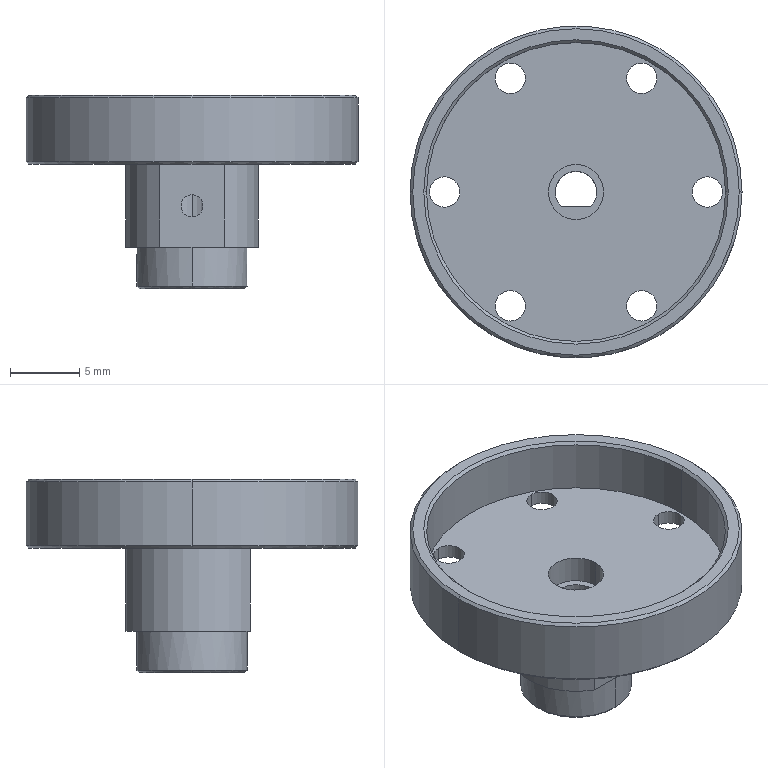NC program | NX | posted with a generic post | part box 24 x 24 x 14 mm
Lines 1710 to 3647 of 3647, first 1767 of 1928 lines:
(ZLEVEL_PROFILE_COPY , TOOL : D1)
N3370 T23 M6
N3372 G54
N3374 G17 G0 G90 X-0.033 Y-0.35 S9500 M3
N3376 G43 Z30. H23
N3378 Z-0.1
N3380 G94 G1 X0.054 Y-0.5 F800.
N3382 X0.07 Y-0.534
N3384 X0.103 Y-0.553
N3386 X0.14 Y-0.55
N3388 X0.835
N3390 G3 X0.979 Y0.202 R1.
N3392 G1 X0.975 Y0.239
N3394 X0.95 Y0.268
N3396 X0.913 Y0.276
N3398 X0.725 Y0.339
N3400 G0 X-0.033 Y-0.35 Z-0.2
N3402 G1 X0.054 Y-0.5
N3404 X0.07 Y-0.534
N3406 X0.103 Y-0.553
N3408 X0.14 Y-0.55
N3410 X0.835
N3412 G3 X0.979 Y0.202 R1.
N3414 G1 X0.975 Y0.239
N3416 X0.95 Y0.268
N3418 X0.913 Y0.276
N3420 X0.725 Y0.339
N3422 G0 X-0.033 Y-0.35 Z-0.3
N3424 G1 X0.054 Y-0.5
N3426 X0.07 Y-0.534
N3428 X0.103 Y-0.553
N3430 X0.14 Y-0.55
N3432 X0.835
N3434 G3 X0.979 Y0.202 R1.
N3436 G1 X0.975 Y0.239
N3438 X0.95 Y0.268
N3440 X0.913 Y0.276
N3442 X0.725 Y0.339
N3444 G0 X-0.033 Y-0.35 Z-0.4
N3446 G1 X0.054 Y-0.5
N3448 X0.07 Y-0.534
N3450 X0.103 Y-0.553
N3452 X0.14 Y-0.55
N3454 X0.835
N3456 G3 X0.979 Y0.202 R1.
N3458 G1 X0.975 Y0.239
N3460 X0.95 Y0.268
N3462 X0.913 Y0.276
N3464 X0.725 Y0.339
N3466 G0 X-0.033 Y-0.35 Z-0.5
N3468 G1 X0.054 Y-0.5
N3470 X0.07 Y-0.534
N3472 X0.103 Y-0.553
N3474 X0.14 Y-0.55
N3476 X0.835
N3478 G3 X0.979 Y0.202 R1.
N3480 G1 X0.975 Y0.239
N3482 X0.95 Y0.268
N3484 X0.913 Y0.276
N3486 X0.725 Y0.339
N3488 G0 X-0.033 Y-0.35 Z-0.6
N3490 G1 X0.054 Y-0.5
N3492 X0.07 Y-0.534
N3494 X0.103 Y-0.553
N3496 X0.14 Y-0.55
N3498 X0.835
N3500 G3 X0.979 Y0.202 R1.
N3502 G1 X0.975 Y0.239
N3504 X0.95 Y0.268
N3506 X0.913 Y0.276
N3508 X0.725 Y0.339
N3510 G0 X-0.033 Y-0.35 Z-0.7
N3512 G1 X0.054 Y-0.5
N3514 X0.07 Y-0.534
N3516 X0.103 Y-0.553
N3518 X0.14 Y-0.55
N3520 X0.835
N3522 G3 X0.979 Y0.202 R1.
N3524 G1 X0.975 Y0.239
N3526 X0.95 Y0.268
N3528 X0.913 Y0.276
N3530 X0.725 Y0.339
N3532 G0 X-0.033 Y-0.35 Z-0.8
N3534 G1 X0.054 Y-0.5
N3536 X0.07 Y-0.534
N3538 X0.103 Y-0.553
N3540 X0.14 Y-0.55
N3542 X0.835
N3544 G3 X0.979 Y0.202 R1.
N3546 G1 X0.975 Y0.239
N3548 X0.95 Y0.268
N3550 X0.913 Y0.276
N3552 X0.725 Y0.339
N3554 G0 X-0.033 Y-0.35 Z-0.9
N3556 G1 X0.054 Y-0.5
N3558 X0.07 Y-0.534
N3560 X0.103 Y-0.553
N3562 X0.14 Y-0.55
N3564 X0.835
N3566 G3 X0.979 Y0.202 R1.
N3568 G1 X0.975 Y0.239
N3570 X0.95 Y0.268
N3572 X0.913 Y0.276
N3574 X0.725 Y0.339
N3576 G0 X-0.033 Y-0.35 Z-1.
N3578 G1 X0.054 Y-0.5
N3580 X0.07 Y-0.534
N3582 X0.103 Y-0.553
N3584 X0.14 Y-0.55
N3586 X0.835
N3588 G3 X0.979 Y0.202 R1.
N3590 G1 X0.975 Y0.239
N3592 X0.95 Y0.268
N3594 X0.913 Y0.276
N3596 X0.725 Y0.339
N3598 G0 X-0.033 Y-0.35 Z-1.1
N3600 G1 X0.054 Y-0.5
N3602 X0.07 Y-0.534
N3604 X0.103 Y-0.553
N3606 X0.14 Y-0.55
N3608 X0.835
N3610 G3 X0.979 Y0.202 R1.
N3612 G1 X0.975 Y0.239
N3614 X0.95 Y0.268
N3616 X0.913 Y0.276
N3618 X0.725 Y0.339
N3620 G0 X-0.033 Y-0.35 Z-1.2
N3622 G1 X0.054 Y-0.5
N3624 X0.07 Y-0.534
N3626 X0.103 Y-0.553
N3628 X0.14 Y-0.55
N3630 X0.835
N3632 G3 X0.979 Y0.202 R1.
N3634 G1 X0.975 Y0.239
N3636 X0.95 Y0.268
N3638 X0.913 Y0.276
N3640 X0.725 Y0.339
N3642 G0 X-0.033 Y-0.35 Z-1.3
N3644 G1 X0.054 Y-0.5
N3646 X0.07 Y-0.534
N3648 X0.103 Y-0.553
N3650 X0.14 Y-0.55
N3652 X0.835
N3654 G3 X0.979 Y0.202 R1.
N3656 G1 X0.975 Y0.239
N3658 X0.95 Y0.268
N3660 X0.913 Y0.276
N3662 X0.725 Y0.339
N3664 G0 X-0.033 Y-0.35 Z-1.4
N3666 G1 X0.054 Y-0.5
N3668 X0.07 Y-0.534
N3670 X0.103 Y-0.553
N3672 X0.14 Y-0.55
N3674 X0.835
N3676 G3 X0.979 Y0.202 R1.
N3678 G1 X0.975 Y0.239
N3680 X0.95 Y0.268
N3682 X0.913 Y0.276
N3684 X0.725 Y0.339
N3686 G0 X-0.033 Y-0.35 Z-1.5
N3688 G1 X0.054 Y-0.5
N3690 X0.07 Y-0.534
N3692 X0.103 Y-0.553
N3694 X0.14 Y-0.55
N3696 X0.835
N3698 G3 X0.979 Y0.202 R1.
N3700 G1 X0.975 Y0.239
N3702 X0.95 Y0.268
N3704 X0.913 Y0.276
N3706 X0.725 Y0.339
N3708 G0 X-0.033 Y-0.35 Z-1.6
N3710 G1 X0.054 Y-0.5
N3712 X0.07 Y-0.534
N3714 X0.103 Y-0.553
N3716 X0.14 Y-0.55
N3718 X0.835
N3720 G3 X0.979 Y0.202 R1.
N3722 G1 X0.975 Y0.239
N3724 X0.95 Y0.268
N3726 X0.913 Y0.276
N3728 X0.725 Y0.339
N3730 G0 X-0.033 Y-0.35 Z-1.7
N3732 G1 X0.054 Y-0.5
N3734 X0.07 Y-0.534
N3736 X0.103 Y-0.553
N3738 X0.14 Y-0.55
N3740 X0.835
N3742 G3 X0.979 Y0.202 R1.
N3744 G1 X0.975 Y0.239
N3746 X0.95 Y0.268
N3748 X0.913 Y0.276
N3750 X0.725 Y0.339
N3752 G0 X-0.033 Y-0.35 Z-1.8
N3754 G1 X0.054 Y-0.5
N3756 X0.07 Y-0.534
N3758 X0.103 Y-0.553
N3760 X0.14 Y-0.55
N3762 X0.835
N3764 G3 X0.979 Y0.202 R1.
N3766 G1 X0.975 Y0.239
N3768 X0.95 Y0.268
N3770 X0.913 Y0.276
N3772 X0.725 Y0.339
N3774 G0 X-0.033 Y-0.35 Z-1.9
N3776 G1 X0.054 Y-0.5
N3778 X0.07 Y-0.534
N3780 X0.103 Y-0.553
N3782 X0.14 Y-0.55
N3784 X0.835
N3786 G3 X0.979 Y0.202 R1.
N3788 G1 X0.975 Y0.239
N3790 X0.95 Y0.268
N3792 X0.913 Y0.276
N3794 X0.725 Y0.339
N3796 G0 X-0.033 Y-0.35 Z-2.
N3798 G1 X0.054 Y-0.5
N3800 X0.07 Y-0.534
N3802 X0.103 Y-0.553
N3804 X0.14 Y-0.55
N3806 X0.835
N3808 G3 X0.979 Y0.202 R1.
N3810 G1 X0.975 Y0.239
N3812 X0.95 Y0.268
N3814 X0.913 Y0.276
N3816 X0.725 Y0.339
N3818 G0 X-0.033 Y-0.35 Z-2.1
N3820 G1 X0.054 Y-0.5
N3822 X0.07 Y-0.534
N3824 X0.103 Y-0.553
N3826 X0.14 Y-0.55
N3828 X0.835
N3830 G3 X0.979 Y0.202 R1.
N3832 G1 X0.975 Y0.239
N3834 X0.95 Y0.268
N3836 X0.913 Y0.276
N3838 X0.725 Y0.339
N3840 G0 X-0.033 Y-0.35 Z-2.2
N3842 G1 X0.054 Y-0.5
N3844 X0.07 Y-0.534
N3846 X0.103 Y-0.553
N3848 X0.14 Y-0.55
N3850 X0.835
N3852 G3 X0.979 Y0.202 R1.
N3854 G1 X0.975 Y0.239
N3856 X0.95 Y0.268
N3858 X0.913 Y0.276
N3860 X0.725 Y0.339
N3862 G0 X-0.033 Y-0.35 Z-2.3
N3864 G1 X0.054 Y-0.5
N3866 X0.07 Y-0.534
N3868 X0.103 Y-0.553
N3870 X0.14 Y-0.55
N3872 X0.835
N3874 G3 X0.979 Y0.202 R1.
N3876 G1 X0.975 Y0.239
N3878 X0.95 Y0.268
N3880 X0.913 Y0.276
N3882 X0.725 Y0.339
N3884 G0 X-0.033 Y-0.35 Z-2.4
N3886 G1 X0.054 Y-0.5
N3888 X0.07 Y-0.534
N3890 X0.103 Y-0.553
N3892 X0.14 Y-0.55
N3894 X0.835
N3896 G3 X0.979 Y0.202 R1.
N3898 G1 X0.975 Y0.239
N3900 X0.95 Y0.268
N3902 X0.913 Y0.276
N3904 X0.725 Y0.339
N3906 G0 X-0.033 Y-0.35 Z-2.5
N3908 G1 X0.054 Y-0.5
N3910 X0.07 Y-0.534
N3912 X0.103 Y-0.553
N3914 X0.14 Y-0.55
N3916 X0.835
N3918 G3 X0.979 Y0.202 R1.
N3920 G1 X0.975 Y0.239
N3922 X0.95 Y0.268
N3924 X0.913 Y0.276
N3926 X0.725 Y0.339
N3928 G0 X-0.033 Y-0.35 Z-2.6
N3930 G1 X0.054 Y-0.5
N3932 X0.07 Y-0.534
N3934 X0.103 Y-0.553
N3936 X0.14 Y-0.55
N3938 X0.835
N3940 G3 X0.979 Y0.202 R1.
N3942 G1 X0.975 Y0.239
N3944 X0.95 Y0.268
N3946 X0.913 Y0.276
N3948 X0.725 Y0.339
N3950 G0 X-0.033 Y-0.35 Z-2.7
N3952 G1 X0.054 Y-0.5
N3954 X0.07 Y-0.534
N3956 X0.103 Y-0.553
N3958 X0.14 Y-0.55
N3960 X0.835
N3962 G3 X0.979 Y0.202 R1.
N3964 G1 X0.975 Y0.239
N3966 X0.95 Y0.268
N3968 X0.913 Y0.276
N3970 X0.725 Y0.339
N3972 G0 X-0.033 Y-0.35 Z-2.8
N3974 G1 X0.054 Y-0.5
N3976 X0.07 Y-0.534
N3978 X0.103 Y-0.553
N3980 X0.14 Y-0.55
N3982 X0.835
N3984 G3 X0.979 Y0.202 R1.
N3986 G1 X0.975 Y0.239
N3988 X0.95 Y0.268
N3990 X0.913 Y0.276
N3992 X0.725 Y0.339
N3994 G0 X-0.033 Y-0.35 Z-2.9
N3996 G1 X0.054 Y-0.5
N3998 X0.07 Y-0.534
N4000 X0.103 Y-0.553
N4002 X0.14 Y-0.55
N4004 X0.835
N4006 G3 X0.979 Y0.202 R1.
N4008 G1 X0.975 Y0.239
N4010 X0.95 Y0.268
N4012 X0.913 Y0.276
N4014 X0.725 Y0.339
N4016 G0 X-0.033 Y-0.35 Z-3.
N4018 G1 X0.054 Y-0.5
N4020 X0.07 Y-0.534
N4022 X0.103 Y-0.553
N4024 X0.14 Y-0.55
N4026 X0.835
N4028 G3 X0.979 Y0.202 R1.
N4030 G1 X0.975 Y0.239
N4032 X0.95 Y0.268
N4034 X0.913 Y0.276
N4036 X0.725 Y0.339
N4038 G0 X-0.033 Y-0.35 Z-3.1
N4040 G1 X0.054 Y-0.5
N4042 X0.07 Y-0.534
N4044 X0.103 Y-0.553
N4046 X0.14 Y-0.55
N4048 X0.835
N4050 G3 X0.979 Y0.202 R1.
N4052 G1 X0.975 Y0.239
N4054 X0.95 Y0.268
N4056 X0.913 Y0.276
N4058 X0.725 Y0.339
N4060 G0 X-0.033 Y-0.35 Z-3.2
N4062 G1 X0.054 Y-0.5
N4064 X0.07 Y-0.534
N4066 X0.103 Y-0.553
N4068 X0.14 Y-0.55
N4070 X0.835
N4072 G3 X0.979 Y0.202 R1.
N4074 G1 X0.975 Y0.239
N4076 X0.95 Y0.268
N4078 X0.913 Y0.276
N4080 X0.725 Y0.339
N4082 G0 X-0.033 Y-0.35 Z-3.3
N4084 G1 X0.054 Y-0.5
N4086 X0.07 Y-0.534
N4088 X0.103 Y-0.553
N4090 X0.14 Y-0.55
N4092 X0.835
N4094 G3 X0.979 Y0.202 R1.
N4096 G1 X0.975 Y0.239
N4098 X0.95 Y0.268
N4100 X0.913 Y0.276
N4102 X0.725 Y0.339
N4104 G0 X-0.033 Y-0.35 Z-3.4
N4106 G1 X0.054 Y-0.5
N4108 X0.07 Y-0.534
N4110 X0.103 Y-0.553
N4112 X0.14 Y-0.55
N4114 X0.835
N4116 G3 X0.979 Y0.202 R1.
N4118 G1 X0.975 Y0.239
N4120 X0.95 Y0.268
N4122 X0.913 Y0.276
N4124 X0.725 Y0.339
N4126 G0 X-0.033 Y-0.35 Z-3.5
N4128 G1 X0.054 Y-0.5
N4130 X0.07 Y-0.534
N4132 X0.103 Y-0.553
N4134 X0.14 Y-0.55
N4136 X0.835
N4138 G3 X0.979 Y0.202 R1.
N4140 G1 X0.975 Y0.239
N4142 X0.95 Y0.268
N4144 X0.913 Y0.276
N4146 X0.725 Y0.339
N4148 G0 X-0.033 Y-0.35 Z-3.6
N4150 G1 X0.054 Y-0.5
N4152 X0.07 Y-0.534
N4154 X0.103 Y-0.553
N4156 X0.14 Y-0.55
N4158 X0.835
N4160 G3 X0.979 Y0.202 R1.
N4162 G1 X0.975 Y0.239
N4164 X0.95 Y0.268
N4166 X0.913 Y0.276
N4168 X0.725 Y0.339
N4170 G0 X-0.033 Y-0.35 Z-3.7
N4172 G1 X0.054 Y-0.5
N4174 X0.07 Y-0.534
N4176 X0.103 Y-0.553
N4178 X0.14 Y-0.55
N4180 X0.835
N4182 G3 X0.979 Y0.202 R1.
N4184 G1 X0.975 Y0.239
N4186 X0.95 Y0.268
N4188 X0.913 Y0.276
N4190 X0.725 Y0.339
N4192 G0 X-0.033 Y-0.35 Z-3.8
N4194 G1 X0.054 Y-0.5
N4196 X0.07 Y-0.534
N4198 X0.103 Y-0.553
N4200 X0.14 Y-0.55
N4202 X0.835
N4204 G3 X0.979 Y0.202 R1.
N4206 G1 X0.975 Y0.239
N4208 X0.95 Y0.268
N4210 X0.913 Y0.276
N4212 X0.725 Y0.339
N4214 G0 X-0.033 Y-0.35 Z-3.9
N4216 G1 X0.054 Y-0.5
N4218 X0.07 Y-0.534
N4220 X0.103 Y-0.553
N4222 X0.14 Y-0.55
N4224 X0.835
N4226 G3 X0.979 Y0.202 R1.
N4228 G1 X0.975 Y0.239
N4230 X0.95 Y0.268
N4232 X0.913 Y0.276
N4234 X0.725 Y0.339
N4236 G0 X-0.033 Y-0.35 Z-4.
N4238 G1 X0.054 Y-0.5
N4240 X0.07 Y-0.534
N4242 X0.103 Y-0.553
N4244 X0.14 Y-0.55
N4246 X0.835
N4248 G3 X0.979 Y0.202 R1.
N4250 G1 X0.975 Y0.239
N4252 X0.95 Y0.268
N4254 X0.913 Y0.276
N4256 X0.725 Y0.339
N4258 G0 X-0.033 Y-0.35 Z-4.1
N4260 G1 X0.054 Y-0.5
N4262 X0.07 Y-0.534
N4264 X0.103 Y-0.553
N4266 X0.14 Y-0.55
N4268 X0.835
N4270 G3 X0.979 Y0.202 R1.
N4272 G1 X0.975 Y0.239
N4274 X0.95 Y0.268
N4276 X0.913 Y0.276
N4278 X0.725 Y0.339
N4280 G0 X-0.033 Y-0.35 Z-4.2
N4282 G1 X0.054 Y-0.5
N4284 X0.07 Y-0.534
N4286 X0.103 Y-0.553
N4288 X0.14 Y-0.55
N4290 X0.835
N4292 G3 X0.979 Y0.202 R1.
N4294 G1 X0.975 Y0.239
N4296 X0.95 Y0.268
N4298 X0.913 Y0.276
N4300 X0.725 Y0.339
N4302 G0 X-0.033 Y-0.35 Z-4.3
N4304 G1 X0.054 Y-0.5
N4306 X0.07 Y-0.534
N4308 X0.103 Y-0.553
N4310 X0.14 Y-0.55
N4312 X0.835
N4314 G3 X0.979 Y0.202 R1.
N4316 G1 X0.975 Y0.239
N4318 X0.95 Y0.268
N4320 X0.913 Y0.276
N4322 X0.725 Y0.339
N4324 G0 X-0.033 Y-0.35 Z-4.4
N4326 G1 X0.054 Y-0.5
N4328 X0.07 Y-0.534
N4330 X0.103 Y-0.553
N4332 X0.14 Y-0.55
N4334 X0.835
N4336 G3 X0.979 Y0.202 R1.
N4338 G1 X0.975 Y0.239
N4340 X0.95 Y0.268
N4342 X0.913 Y0.276
N4344 X0.725 Y0.339
N4346 G0 X-0.033 Y-0.35 Z-4.5
N4348 G1 X0.054 Y-0.5
N4350 X0.07 Y-0.534
N4352 X0.103 Y-0.553
N4354 X0.14 Y-0.55
N4356 X0.835
N4358 G3 X0.979 Y0.202 R1.
N4360 G1 X0.975 Y0.239
N4362 X0.95 Y0.268
N4364 X0.913 Y0.276
N4366 X0.725 Y0.339
N4368 G0 X-0.033 Y-0.35 Z-4.6
N4370 G1 X0.054 Y-0.5
N4372 X0.07 Y-0.534
N4374 X0.103 Y-0.553
N4376 X0.14 Y-0.55
N4378 X0.835
N4380 G3 X0.979 Y0.202 R1.
N4382 G1 X0.975 Y0.239
N4384 X0.95 Y0.268
N4386 X0.913 Y0.276
N4388 X0.725 Y0.339
N4390 G0 X-0.033 Y-0.35 Z-4.7
N4392 G1 X0.054 Y-0.5
N4394 X0.07 Y-0.534
N4396 X0.103 Y-0.553
N4398 X0.14 Y-0.55
N4400 X0.835
N4402 G3 X0.979 Y0.202 R1.
N4404 G1 X0.975 Y0.239
N4406 X0.95 Y0.268
N4408 X0.913 Y0.276
N4410 X0.725 Y0.339
N4412 G0 X-0.033 Y-0.35 Z-4.8
N4414 G1 X0.054 Y-0.5
N4416 X0.07 Y-0.534
N4418 X0.103 Y-0.553
N4420 X0.14 Y-0.55
N4422 X0.835
N4424 G3 X0.979 Y0.202 R1.
N4426 G1 X0.975 Y0.239
N4428 X0.95 Y0.268
N4430 X0.913 Y0.276
N4432 X0.725 Y0.339
N4434 G0 X-0.033 Y-0.35 Z-4.9
N4436 G1 X0.054 Y-0.5
N4438 X0.07 Y-0.534
N4440 X0.103 Y-0.553
N4442 X0.14 Y-0.55
N4444 X0.835
N4446 G3 X0.979 Y0.202 R1.
N4448 G1 X0.975 Y0.239
N4450 X0.95 Y0.268
N4452 X0.913 Y0.276
N4454 X0.725 Y0.339
N4456 G0 X-0.033 Y-0.35 Z-5.
N4458 G1 X0.054 Y-0.5
N4460 X0.07 Y-0.534
N4462 X0.103 Y-0.553
N4464 X0.14 Y-0.55
N4466 X0.835
N4468 G3 X0.979 Y0.202 R1.
N4470 G1 X0.975 Y0.239
N4472 X0.95 Y0.268
N4474 X0.913 Y0.276
N4476 X0.725 Y0.339
N4478 G0 X-0.033 Y-0.35 Z-5.1
N4480 G1 X0.054 Y-0.5
N4482 X0.07 Y-0.534
N4484 X0.103 Y-0.553
N4486 X0.14 Y-0.55
N4488 X0.835
N4490 G3 X0.979 Y0.202 R1.
N4492 G1 X0.975 Y0.239
N4494 X0.95 Y0.268
N4496 X0.913 Y0.276
N4498 X0.725 Y0.339
N4500 G0 X-0.033 Y-0.35 Z-5.2
N4502 G1 X0.054 Y-0.5
N4504 X0.07 Y-0.534
N4506 X0.103 Y-0.553
N4508 X0.14 Y-0.55
N4510 X0.835
N4512 G3 X0.979 Y0.202 R1.
N4514 G1 X0.975 Y0.239
N4516 X0.95 Y0.268
N4518 X0.913 Y0.276
N4520 X0.725 Y0.339
N4522 G0 X-0.033 Y-0.35 Z-5.3
N4524 G1 X0.054 Y-0.5
N4526 X0.07 Y-0.534
N4528 X0.103 Y-0.553
N4530 X0.14 Y-0.55
N4532 X0.835
N4534 G3 X0.979 Y0.202 R1.
N4536 G1 X0.975 Y0.239
N4538 X0.95 Y0.268
N4540 X0.913 Y0.276
N4542 X0.725 Y0.339
N4544 G0 X-0.033 Y-0.35 Z-5.4
N4546 G1 X0.054 Y-0.5
N4548 X0.07 Y-0.534
N4550 X0.103 Y-0.553
N4552 X0.14 Y-0.55
N4554 X0.835
N4556 G3 X0.979 Y0.202 R1.
N4558 G1 X0.975 Y0.239
N4560 X0.95 Y0.268
N4562 X0.913 Y0.276
N4564 X0.725 Y0.339
N4566 G0 X-0.033 Y-0.35 Z-5.5
N4568 G1 X0.054 Y-0.5
N4570 X0.07 Y-0.534
N4572 X0.103 Y-0.553
N4574 X0.14 Y-0.55
N4576 X0.835
N4578 G3 X0.979 Y0.202 R1.
N4580 G1 X0.975 Y0.239
N4582 X0.95 Y0.268
N4584 X0.913 Y0.276
N4586 X0.725 Y0.339
N4588 G0 X-0.033 Y-0.35 Z-5.6
N4590 G1 X0.054 Y-0.5
N4592 X0.07 Y-0.534
N4594 X0.103 Y-0.553
N4596 X0.14 Y-0.55
N4598 X0.835
N4600 G3 X0.979 Y0.202 R1.
N4602 G1 X0.975 Y0.239
N4604 X0.95 Y0.268
N4606 X0.913 Y0.276
N4608 X0.725 Y0.339
N4610 G0 X-0.033 Y-0.35 Z-5.7
N4612 G1 X0.054 Y-0.5
N4614 X0.07 Y-0.534
N4616 X0.103 Y-0.553
N4618 X0.14 Y-0.55
N4620 X0.835
N4622 G3 X0.979 Y0.202 R1.
N4624 G1 X0.975 Y0.239
N4626 X0.95 Y0.268
N4628 X0.913 Y0.276
N4630 X0.725 Y0.339
N4632 G0 X-0.033 Y-0.35 Z-5.8
N4634 G1 X0.054 Y-0.5
N4636 X0.07 Y-0.534
N4638 X0.103 Y-0.553
N4640 X0.14 Y-0.55
N4642 X0.835
N4644 G3 X0.979 Y0.202 R1.
N4646 G1 X0.975 Y0.239
N4648 X0.95 Y0.268
N4650 X0.913 Y0.276
N4652 X0.725 Y0.339
N4654 G0 X-0.033 Y-0.35 Z-5.9
N4656 G1 X0.054 Y-0.5
N4658 X0.07 Y-0.534
N4660 X0.103 Y-0.553
N4662 X0.14 Y-0.55
N4664 X0.835
N4666 G3 X0.979 Y0.202 R1.
N4668 G1 X0.975 Y0.239
N4670 X0.95 Y0.268
N4672 X0.913 Y0.276
N4674 X0.725 Y0.339
N4676 G0 X-0.033 Y-0.35 Z-6.
N4678 G1 X0.054 Y-0.5
N4680 X0.07 Y-0.534
N4682 X0.103 Y-0.553
N4684 X0.14 Y-0.55
N4686 X0.835
N4688 G3 X0.979 Y0.202 R1.
N4690 G1 X0.975 Y0.239
N4692 X0.95 Y0.268
N4694 X0.913 Y0.276
N4696 X0.725 Y0.339
N4698 G0 X-0.033 Y-0.35 Z-6.1
N4700 G1 X0.054 Y-0.5
N4702 X0.07 Y-0.534
N4704 X0.103 Y-0.553
N4706 X0.14 Y-0.55
N4708 X0.835
N4710 G3 X0.979 Y0.202 R1.
N4712 G1 X0.975 Y0.239
N4714 X0.95 Y0.268
N4716 X0.913 Y0.276
N4718 X0.725 Y0.339
N4720 G0 X-0.033 Y-0.35 Z-6.2
N4722 G1 X0.054 Y-0.5
N4724 X0.07 Y-0.534
N4726 X0.103 Y-0.553
N4728 X0.14 Y-0.55
N4730 X0.835
N4732 G3 X0.979 Y0.202 R1.
N4734 G1 X0.975 Y0.239
N4736 X0.95 Y0.268
N4738 X0.913 Y0.276
N4740 X0.725 Y0.339
N4742 G0 X-0.033 Y-0.35 Z-6.3
N4744 G1 X0.054 Y-0.5
N4746 X0.07 Y-0.534
N4748 X0.103 Y-0.553
N4750 X0.14 Y-0.55
N4752 X0.835
N4754 G3 X0.979 Y0.202 R1.
N4756 G1 X0.975 Y0.239
N4758 X0.95 Y0.268
N4760 X0.913 Y0.276
N4762 X0.725 Y0.339
N4764 G0 X-0.033 Y-0.35 Z-6.4
N4766 G1 X0.054 Y-0.5
N4768 X0.07 Y-0.534
N4770 X0.103 Y-0.553
N4772 X0.14 Y-0.55
N4774 X0.835
N4776 G3 X0.979 Y0.202 R1.
N4778 G1 X0.975 Y0.239
N4780 X0.95 Y0.268
N4782 X0.913 Y0.276
N4784 X0.725 Y0.339
N4786 G0 X-0.033 Y-0.35 Z-6.5
N4788 G1 X0.054 Y-0.5
N4790 X0.07 Y-0.534
N4792 X0.103 Y-0.553
N4794 X0.14 Y-0.55
N4796 X0.835
N4798 G3 X0.979 Y0.202 R1.
N4800 G1 X0.975 Y0.239
N4802 X0.95 Y0.268
N4804 X0.913 Y0.276
N4806 X0.725 Y0.339
N4808 G0 X-0.033 Y-0.35 Z-6.6
N4810 G1 X0.054 Y-0.5
N4812 X0.07 Y-0.534
N4814 X0.103 Y-0.553
N4816 X0.14 Y-0.55
N4818 X0.835
N4820 G3 X0.979 Y0.202 R1.
N4822 G1 X0.975 Y0.239
N4824 X0.95 Y0.268
N4826 X0.913 Y0.276
N4828 X0.725 Y0.339
N4830 G0 X-0.033 Y-0.35 Z-6.7
N4832 G1 X0.054 Y-0.5
N4834 X0.07 Y-0.534
N4836 X0.103 Y-0.553
N4838 X0.14 Y-0.55
N4840 X0.835
N4842 G3 X0.979 Y0.202 R1.
N4844 G1 X0.975 Y0.239
N4846 X0.95 Y0.268
N4848 X0.913 Y0.276
N4850 X0.725 Y0.339
N4852 G0 X-0.033 Y-0.35 Z-6.8
N4854 G1 X0.054 Y-0.5
N4856 X0.07 Y-0.534
N4858 X0.103 Y-0.553
N4860 X0.14 Y-0.55
N4862 X0.835
N4864 G3 X0.979 Y0.202 R1.
N4866 G1 X0.975 Y0.239
N4868 X0.95 Y0.268
N4870 X0.913 Y0.276
N4872 X0.725 Y0.339
N4874 G0 X-0.033 Y-0.35 Z-6.9
N4876 G1 X0.054 Y-0.5
N4878 X0.07 Y-0.534
N4880 X0.103 Y-0.553
N4882 X0.14 Y-0.55
N4884 X0.835
N4886 G3 X0.979 Y0.202 R1.
N4888 G1 X0.975 Y0.239
N4890 X0.95 Y0.268
N4892 X0.913 Y0.276
N4894 X0.725 Y0.339
N4896 G0 X-0.033 Y-0.35 Z-7.
N4898 G1 X0.054 Y-0.5
N4900 X0.07 Y-0.534
N4902 X0.103 Y-0.553
N4904 X0.14 Y-0.55
N4906 X0.835
N4908 G3 X0.979 Y0.202 R1.
N4910 G1 X0.975 Y0.239
N4912 X0.95 Y0.268
N4914 X0.913 Y0.276
N4916 X0.725 Y0.339
N4918 G0 X-0.033 Y-0.35 Z-7.1
N4920 G1 X0.054 Y-0.5
N4922 X0.07 Y-0.534
N4924 X0.103 Y-0.553
N4926 X0.14 Y-0.55
N4928 X0.835
N4930 G3 X0.979 Y0.202 R1.
N4932 G1 X0.975 Y0.239
N4934 X0.95 Y0.268
N4936 X0.913 Y0.276
N4938 X0.725 Y0.339
N4940 G0 X-0.033 Y-0.35 Z-7.2
N4942 G1 X0.054 Y-0.5
N4944 X0.07 Y-0.534
N4946 X0.103 Y-0.553
N4948 X0.14 Y-0.55
N4950 X0.835
N4952 G3 X0.979 Y0.202 R1.
N4954 G1 X0.975 Y0.239
N4956 X0.95 Y0.268
N4958 X0.913 Y0.276
N4960 X0.725 Y0.339
N4962 G0 X-0.033 Y-0.35 Z-7.3
N4964 G1 X0.054 Y-0.5
N4966 X0.07 Y-0.534
N4968 X0.103 Y-0.553
N4970 X0.14 Y-0.55
N4972 X0.835
N4974 G3 X0.979 Y0.202 R1.
N4976 G1 X0.975 Y0.239
N4978 X0.95 Y0.268
N4980 X0.913 Y0.276
N4982 X0.725 Y0.339
N4984 G0 X-0.033 Y-0.35 Z-7.4
N4986 G1 X0.054 Y-0.5
N4988 X0.07 Y-0.534
N4990 X0.103 Y-0.553
N4992 X0.14 Y-0.55
N4994 X0.835
N4996 G3 X0.979 Y0.202 R1.
N4998 G1 X0.975 Y0.239
N5000 X0.95 Y0.268
N5002 X0.913 Y0.276
N5004 X0.725 Y0.339
N5006 G0 X-0.033 Y-0.35 Z-7.5
N5008 G1 X0.054 Y-0.5
N5010 X0.07 Y-0.534
N5012 X0.103 Y-0.553
N5014 X0.14 Y-0.55
N5016 X0.835
N5018 G3 X0.979 Y0.202 R1.
N5020 G1 X0.975 Y0.239
N5022 X0.95 Y0.268
N5024 X0.913 Y0.276
N5026 X0.725 Y0.339
N5028 G0 X-0.033 Y-0.35 Z-7.6
N5030 G1 X0.054 Y-0.5
N5032 X0.07 Y-0.534
N5034 X0.103 Y-0.553
N5036 X0.14 Y-0.55
N5038 X0.835
N5040 G3 X0.979 Y0.202 R1.
N5042 G1 X0.975 Y0.239
N5044 X0.95 Y0.268
N5046 X0.913 Y0.276
N5048 X0.725 Y0.339
N5050 G0 X-0.033 Y-0.35 Z-7.7
N5052 G1 X0.054 Y-0.5
N5054 X0.07 Y-0.534
N5056 X0.103 Y-0.553
N5058 X0.14 Y-0.55
N5060 X0.835
N5062 G3 X0.979 Y0.202 R1.
N5064 G1 X0.975 Y0.239
N5066 X0.95 Y0.268
N5068 X0.913 Y0.276
N5070 X0.725 Y0.339
N5072 G0 X-0.033 Y-0.35 Z-7.8
N5074 G1 X0.054 Y-0.5
N5076 X0.07 Y-0.534
N5078 X0.103 Y-0.553
N5080 X0.14 Y-0.55
N5082 X0.835
N5084 G3 X0.979 Y0.202 R1.
N5086 G1 X0.975 Y0.239
N5088 X0.95 Y0.268
N5090 X0.913 Y0.276
N5092 X0.725 Y0.339
N5094 G0 X-0.033 Y-0.35 Z-7.9
N5096 G1 X0.054 Y-0.5
N5098 X0.07 Y-0.534
N5100 X0.103 Y-0.553
N5102 X0.14 Y-0.55
N5104 X0.835
N5106 G3 X0.979 Y0.202 R1.
N5108 G1 X0.975 Y0.239
N5110 X0.95 Y0.268
N5112 X0.913 Y0.276
N5114 X0.725 Y0.339
N5116 G0 X-0.033 Y-0.35 Z-8.
N5118 G1 X0.054 Y-0.5
N5120 X0.07 Y-0.534
N5122 X0.103 Y-0.553
N5124 X0.14 Y-0.55
N5126 X0.835
N5128 G3 X0.979 Y0.202 R1.
N5130 G1 X0.975 Y0.239
N5132 X0.95 Y0.268
N5134 X0.913 Y0.276
N5136 X0.725 Y0.339
N5138 G0 Z30.
N5140 X-0.725
N5142 Z-0.1
N5144 G1 X-0.913 Y0.276
N5146 X-0.95 Y0.268
N5148 X-0.975 Y0.239
N5150 X-0.979 Y0.202
N5152 G3 X-0.835 Y-0.55 R1.
N5154 G1 X-0.14
N5156 X-0.103 Y-0.553
N5158 X-0.07 Y-0.534
N5160 X-0.054 Y-0.5
N5162 X0.033 Y-0.35
N5164 G0 X-0.725 Y0.339 Z-0.2
N5166 G1 X-0.913 Y0.276
N5168 X-0.95 Y0.268
N5170 X-0.975 Y0.239
N5172 X-0.979 Y0.202
N5174 G3 X-0.835 Y-0.55 R1.
N5176 G1 X-0.14
N5178 X-0.103 Y-0.553
N5180 X-0.07 Y-0.534
N5182 X-0.054 Y-0.5
N5184 X0.033 Y-0.35
N5186 G0 X-0.725 Y0.339 Z-0.3
N5188 G1 X-0.913 Y0.276
N5190 X-0.95 Y0.268
N5192 X-0.975 Y0.239
N5194 X-0.979 Y0.202
N5196 G3 X-0.835 Y-0.55 R1.
N5198 G1 X-0.14
N5200 X-0.103 Y-0.553
N5202 X-0.07 Y-0.534
N5204 X-0.054 Y-0.5
N5206 X0.033 Y-0.35
N5208 G0 X-0.725 Y0.339 Z-0.4
N5210 G1 X-0.913 Y0.276
N5212 X-0.95 Y0.268
N5214 X-0.975 Y0.239
N5216 X-0.979 Y0.202
N5218 G3 X-0.835 Y-0.55 R1.
N5220 G1 X-0.14
N5222 X-0.103 Y-0.553
N5224 X-0.07 Y-0.534
N5226 X-0.054 Y-0.5
N5228 X0.033 Y-0.35
N5230 G0 X-0.725 Y0.339 Z-0.5
N5232 G1 X-0.913 Y0.276
N5234 X-0.95 Y0.268
N5236 X-0.975 Y0.239
N5238 X-0.979 Y0.202
N5240 G3 X-0.835 Y-0.55 R1.
N5242 G1 X-0.14
N5244 X-0.103 Y-0.553
N5246 X-0.07 Y-0.534
N5248 X-0.054 Y-0.5
N5250 X0.033 Y-0.35
N5252 G0 X-0.725 Y0.339 Z-0.6
N5254 G1 X-0.913 Y0.276
N5256 X-0.95 Y0.268
N5258 X-0.975 Y0.239
N5260 X-0.979 Y0.202
N5262 G3 X-0.835 Y-0.55 R1.
N5264 G1 X-0.14
N5266 X-0.103 Y-0.553
N5268 X-0.07 Y-0.534
N5270 X-0.054 Y-0.5
N5272 X0.033 Y-0.35
N5274 G0 X-0.725 Y0.339 Z-0.7
N5276 G1 X-0.913 Y0.276
N5278 X-0.95 Y0.268
N5280 X-0.975 Y0.239
N5282 X-0.979 Y0.202
N5284 G3 X-0.835 Y-0.55 R1.
N5286 G1 X-0.14
N5288 X-0.103 Y-0.553
N5290 X-0.07 Y-0.534
N5292 X-0.054 Y-0.5
N5294 X0.033 Y-0.35
N5296 G0 X-0.725 Y0.339 Z-0.8
N5298 G1 X-0.913 Y0.276
N5300 X-0.95 Y0.268
N5302 X-0.975 Y0.239
N5304 X-0.979 Y0.202
N5306 G3 X-0.835 Y-0.55 R1.
N5308 G1 X-0.14
N5310 X-0.103 Y-0.553
N5312 X-0.07 Y-0.534
N5314 X-0.054 Y-0.5
N5316 X0.033 Y-0.35
N5318 G0 X-0.725 Y0.339 Z-0.9
N5320 G1 X-0.913 Y0.276
N5322 X-0.95 Y0.268
N5324 X-0.975 Y0.239
N5326 X-0.979 Y0.202
N5328 G3 X-0.835 Y-0.55 R1.
N5330 G1 X-0.14
N5332 X-0.103 Y-0.553
N5334 X-0.07 Y-0.534
N5336 X-0.054 Y-0.5
N5338 X0.033 Y-0.35
N5340 G0 X-0.725 Y0.339 Z-1.
N5342 G1 X-0.913 Y0.276
N5344 X-0.95 Y0.268
N5346 X-0.975 Y0.239
N5348 X-0.979 Y0.202
N5350 G3 X-0.835 Y-0.55 R1.
N5352 G1 X-0.14
N5354 X-0.103 Y-0.553
N5356 X-0.07 Y-0.534
N5358 X-0.054 Y-0.5
N5360 X0.033 Y-0.35
N5362 G0 X-0.725 Y0.339 Z-1.1
N5364 G1 X-0.913 Y0.276
N5366 X-0.95 Y0.268
N5368 X-0.975 Y0.239
N5370 X-0.979 Y0.202
N5372 G3 X-0.835 Y-0.55 R1.
N5374 G1 X-0.14
N5376 X-0.103 Y-0.553
N5378 X-0.07 Y-0.534
N5380 X-0.054 Y-0.5
N5382 X0.033 Y-0.35
N5384 G0 X-0.725 Y0.339 Z-1.2
N5386 G1 X-0.913 Y0.276
N5388 X-0.95 Y0.268
N5390 X-0.975 Y0.239
N5392 X-0.979 Y0.202
N5394 G3 X-0.835 Y-0.55 R1.
N5396 G1 X-0.14
N5398 X-0.103 Y-0.553
N5400 X-0.07 Y-0.534
N5402 X-0.054 Y-0.5
N5404 X0.033 Y-0.35
N5406 G0 X-0.725 Y0.339 Z-1.3
N5408 G1 X-0.913 Y0.276
N5410 X-0.95 Y0.268
N5412 X-0.975 Y0.239
N5414 X-0.979 Y0.202
N5416 G3 X-0.835 Y-0.55 R1.
N5418 G1 X-0.14
N5420 X-0.103 Y-0.553
N5422 X-0.07 Y-0.534
N5424 X-0.054 Y-0.5
N5426 X0.033 Y-0.35
N5428 G0 X-0.725 Y0.339 Z-1.4
N5430 G1 X-0.913 Y0.276
N5432 X-0.95 Y0.268
N5434 X-0.975 Y0.239
N5436 X-0.979 Y0.202
N5438 G3 X-0.835 Y-0.55 R1.
N5440 G1 X-0.14
N5442 X-0.103 Y-0.553
N5444 X-0.07 Y-0.534
N5446 X-0.054 Y-0.5
N5448 X0.033 Y-0.35
N5450 G0 X-0.725 Y0.339 Z-1.5
N5452 G1 X-0.913 Y0.276
N5454 X-0.95 Y0.268
N5456 X-0.975 Y0.239
N5458 X-0.979 Y0.202
N5460 G3 X-0.835 Y-0.55 R1.
N5462 G1 X-0.14
N5464 X-0.103 Y-0.553
N5466 X-0.07 Y-0.534
N5468 X-0.054 Y-0.5
N5470 X0.033 Y-0.35
N5472 G0 X-0.725 Y0.339 Z-1.6
N5474 G1 X-0.913 Y0.276
N5476 X-0.95 Y0.268
N5478 X-0.975 Y0.239
N5480 X-0.979 Y0.202
N5482 G3 X-0.835 Y-0.55 R1.
N5484 G1 X-0.14
N5486 X-0.103 Y-0.553
N5488 X-0.07 Y-0.534
N5490 X-0.054 Y-0.5
N5492 X0.033 Y-0.35
N5494 G0 X-0.725 Y0.339 Z-1.7
N5496 G1 X-0.913 Y0.276
N5498 X-0.95 Y0.268
N5500 X-0.975 Y0.239
N5502 X-0.979 Y0.202
N5504 G3 X-0.835 Y-0.55 R1.
N5506 G1 X-0.14
N5508 X-0.103 Y-0.553
N5510 X-0.07 Y-0.534
N5512 X-0.054 Y-0.5
N5514 X0.033 Y-0.35
N5516 G0 X-0.725 Y0.339 Z-1.8
N5518 G1 X-0.913 Y0.276
N5520 X-0.95 Y0.268
N5522 X-0.975 Y0.239
N5524 X-0.979 Y0.202
N5526 G3 X-0.835 Y-0.55 R1.
N5528 G1 X-0.14
N5530 X-0.103 Y-0.553
N5532 X-0.07 Y-0.534
N5534 X-0.054 Y-0.5
N5536 X0.033 Y-0.35
N5538 G0 X-0.725 Y0.339 Z-1.9
N5540 G1 X-0.913 Y0.276
N5542 X-0.95 Y0.268
N5544 X-0.975 Y0.239
N5546 X-0.979 Y0.202
N5548 G3 X-0.835 Y-0.55 R1.
N5550 G1 X-0.14
N5552 X-0.103 Y-0.553
N5554 X-0.07 Y-0.534
N5556 X-0.054 Y-0.5
N5558 X0.033 Y-0.35
N5560 G0 X-0.725 Y0.339 Z-2.
N5562 G1 X-0.913 Y0.276
N5564 X-0.95 Y0.268
N5566 X-0.975 Y0.239
N5568 X-0.979 Y0.202
N5570 G3 X-0.835 Y-0.55 R1.
N5572 G1 X-0.14
N5574 X-0.103 Y-0.553
N5576 X-0.07 Y-0.534
N5578 X-0.054 Y-0.5
N5580 X0.033 Y-0.35
N5582 G0 X-0.725 Y0.339 Z-2.1
N5584 G1 X-0.913 Y0.276
N5586 X-0.95 Y0.268
N5588 X-0.975 Y0.239
N5590 X-0.979 Y0.202
N5592 G3 X-0.835 Y-0.55 R1.
N5594 G1 X-0.14
N5596 X-0.103 Y-0.553
N5598 X-0.07 Y-0.534
N5600 X-0.054 Y-0.5
N5602 X0.033 Y-0.35
N5604 G0 X-0.725 Y0.339 Z-2.2
N5606 G1 X-0.913 Y0.276
N5608 X-0.95 Y0.268
N5610 X-0.975 Y0.239
N5612 X-0.979 Y0.202
N5614 G3 X-0.835 Y-0.55 R1.
N5616 G1 X-0.14
N5618 X-0.103 Y-0.553
N5620 X-0.07 Y-0.534
N5622 X-0.054 Y-0.5
N5624 X0.033 Y-0.35
N5626 G0 X-0.725 Y0.339 Z-2.3
N5628 G1 X-0.913 Y0.276
N5630 X-0.95 Y0.268
N5632 X-0.975 Y0.239
N5634 X-0.979 Y0.202
N5636 G3 X-0.835 Y-0.55 R1.
N5638 G1 X-0.14
N5640 X-0.103 Y-0.553
N5642 X-0.07 Y-0.534
N5644 X-0.054 Y-0.5
N5646 X0.033 Y-0.35
N5648 G0 X-0.725 Y0.339 Z-2.4
N5650 G1 X-0.913 Y0.276
N5652 X-0.95 Y0.268
N5654 X-0.975 Y0.239
N5656 X-0.979 Y0.202
N5658 G3 X-0.835 Y-0.55 R1.
N5660 G1 X-0.14
N5662 X-0.103 Y-0.553
N5664 X-0.07 Y-0.534
N5666 X-0.054 Y-0.5
N5668 X0.033 Y-0.35
N5670 G0 X-0.725 Y0.339 Z-2.5
N5672 G1 X-0.913 Y0.276
N5674 X-0.95 Y0.268
N5676 X-0.975 Y0.239
N5678 X-0.979 Y0.202
N5680 G3 X-0.835 Y-0.55 R1.
N5682 G1 X-0.14
N5684 X-0.103 Y-0.553
N5686 X-0.07 Y-0.534
N5688 X-0.054 Y-0.5
N5690 X0.033 Y-0.35
N5692 G0 X-0.725 Y0.339 Z-2.6
N5694 G1 X-0.913 Y0.276
N5696 X-0.95 Y0.268
N5698 X-0.975 Y0.239
N5700 X-0.979 Y0.202
N5702 G3 X-0.835 Y-0.55 R1.
N5704 G1 X-0.14
N5706 X-0.103 Y-0.553
N5708 X-0.07 Y-0.534
N5710 X-0.054 Y-0.5
N5712 X0.033 Y-0.35
N5714 G0 X-0.725 Y0.339 Z-2.7
N5716 G1 X-0.913 Y0.276
N5718 X-0.95 Y0.268
N5720 X-0.975 Y0.239
N5722 X-0.979 Y0.202
N5724 G3 X-0.835 Y-0.55 R1.
N5726 G1 X-0.14
N5728 X-0.103 Y-0.553
N5730 X-0.07 Y-0.534
N5732 X-0.054 Y-0.5
N5734 X0.033 Y-0.35
N5736 G0 X-0.725 Y0.339 Z-2.8
N5738 G1 X-0.913 Y0.276
N5740 X-0.95 Y0.268
N5742 X-0.975 Y0.239
N5744 X-0.979 Y0.202
N5746 G3 X-0.835 Y-0.55 R1.
N5748 G1 X-0.14
N5750 X-0.103 Y-0.553
N5752 X-0.07 Y-0.534
N5754 X-0.054 Y-0.5
N5756 X0.033 Y-0.35
N5758 G0 X-0.725 Y0.339 Z-2.9
N5760 G1 X-0.913 Y0.276
N5762 X-0.95 Y0.268
N5764 X-0.975 Y0.239
N5766 X-0.979 Y0.202
N5768 G3 X-0.835 Y-0.55 R1.
N5770 G1 X-0.14
N5772 X-0.103 Y-0.553
N5774 X-0.07 Y-0.534
N5776 X-0.054 Y-0.5
N5778 X0.033 Y-0.35
N5780 G0 X-0.725 Y0.339 Z-3.
N5782 G1 X-0.913 Y0.276
N5784 X-0.95 Y0.268
N5786 X-0.975 Y0.239
N5788 X-0.979 Y0.202
N5790 G3 X-0.835 Y-0.55 R1.
N5792 G1 X-0.14
N5794 X-0.103 Y-0.553
N5796 X-0.07 Y-0.534
N5798 X-0.054 Y-0.5
N5800 X0.033 Y-0.35
N5802 G0 X-0.725 Y0.339 Z-3.1
N5804 G1 X-0.913 Y0.276
N5806 X-0.95 Y0.268
N5808 X-0.975 Y0.239
N5810 X-0.979 Y0.202
N5812 G3 X-0.835 Y-0.55 R1.
N5814 G1 X-0.14
N5816 X-0.103 Y-0.553
N5818 X-0.07 Y-0.534
N5820 X-0.054 Y-0.5
N5822 X0.033 Y-0.35
N5824 G0 X-0.725 Y0.339 Z-3.2
N5826 G1 X-0.913 Y0.276
N5828 X-0.95 Y0.268
N5830 X-0.975 Y0.239
N5832 X-0.979 Y0.202
N5834 G3 X-0.835 Y-0.55 R1.
N5836 G1 X-0.14
N5838 X-0.103 Y-0.553
N5840 X-0.07 Y-0.534
N5842 X-0.054 Y-0.5
N5844 X0.033 Y-0.35
N5846 G0 X-0.725 Y0.339 Z-3.3
N5848 G1 X-0.913 Y0.276
N5850 X-0.95 Y0.268
N5852 X-0.975 Y0.239
N5854 X-0.979 Y0.202
N5856 G3 X-0.835 Y-0.55 R1.
N5858 G1 X-0.14
N5860 X-0.103 Y-0.553
N5862 X-0.07 Y-0.534
N5864 X-0.054 Y-0.5
N5866 X0.033 Y-0.35
N5868 G0 X-0.725 Y0.339 Z-3.4
N5870 G1 X-0.913 Y0.276
N5872 X-0.95 Y0.268
N5874 X-0.975 Y0.239
N5876 X-0.979 Y0.202
N5878 G3 X-0.835 Y-0.55 R1.
N5880 G1 X-0.14
N5882 X-0.103 Y-0.553
N5884 X-0.07 Y-0.534
N5886 X-0.054 Y-0.5
N5888 X0.033 Y-0.35
N5890 G0 X-0.725 Y0.339 Z-3.5
N5892 G1 X-0.913 Y0.276
N5894 X-0.95 Y0.268
N5896 X-0.975 Y0.239
N5898 X-0.979 Y0.202
N5900 G3 X-0.835 Y-0.55 R1.
N5902 G1 X-0.14
N5904 X-0.103 Y-0.553
N5906 X-0.07 Y-0.534
N5908 X-0.054 Y-0.5
N5910 X0.033 Y-0.35
N5912 G0 X-0.725 Y0.339 Z-3.6
N5914 G1 X-0.913 Y0.276
N5916 X-0.95 Y0.268
N5918 X-0.975 Y0.239
N5920 X-0.979 Y0.202
N5922 G3 X-0.835 Y-0.55 R1.
N5924 G1 X-0.14
N5926 X-0.103 Y-0.553
N5928 X-0.07 Y-0.534
N5930 X-0.054 Y-0.5
N5932 X0.033 Y-0.35
N5934 G0 X-0.725 Y0.339 Z-3.7
N5936 G1 X-0.913 Y0.276
N5938 X-0.95 Y0.268
N5940 X-0.975 Y0.239
N5942 X-0.979 Y0.202
N5944 G3 X-0.835 Y-0.55 R1.
N5946 G1 X-0.14
N5948 X-0.103 Y-0.553
N5950 X-0.07 Y-0.534
N5952 X-0.054 Y-0.5
N5954 X0.033 Y-0.35
N5956 G0 X-0.725 Y0.339 Z-3.8
N5958 G1 X-0.913 Y0.276
N5960 X-0.95 Y0.268
N5962 X-0.975 Y0.239
N5964 X-0.979 Y0.202
N5966 G3 X-0.835 Y-0.55 R1.
N5968 G1 X-0.14
N5970 X-0.103 Y-0.553
N5972 X-0.07 Y-0.534
N5974 X-0.054 Y-0.5
N5976 X0.033 Y-0.35
N5978 G0 X-0.725 Y0.339 Z-3.9
N5980 G1 X-0.913 Y0.276
N5982 X-0.95 Y0.268
N5984 X-0.975 Y0.239
N5986 X-0.979 Y0.202
N5988 G3 X-0.835 Y-0.55 R1.
N5990 G1 X-0.14
N5992 X-0.103 Y-0.553
N5994 X-0.07 Y-0.534
N5996 X-0.054 Y-0.5
N5998 X0.033 Y-0.35
N6000 G0 X-0.725 Y0.339 Z-4.
N6002 G1 X-0.913 Y0.276
N6004 X-0.95 Y0.268
N6006 X-0.975 Y0.239
N6008 X-0.979 Y0.202
N6010 G3 X-0.835 Y-0.55 R1.
N6012 G1 X-0.14
N6014 X-0.103 Y-0.553
N6016 X-0.07 Y-0.534
N6018 X-0.054 Y-0.5
N6020 X0.033 Y-0.35
N6022 G0 X-0.725 Y0.339 Z-4.1
N6024 G1 X-0.913 Y0.276
N6026 X-0.95 Y0.268
N6028 X-0.975 Y0.239
N6030 X-0.979 Y0.202
N6032 G3 X-0.835 Y-0.55 R1.
N6034 G1 X-0.14
N6036 X-0.103 Y-0.553
N6038 X-0.07 Y-0.534
N6040 X-0.054 Y-0.5
N6042 X0.033 Y-0.35
N6044 G0 X-0.725 Y0.339 Z-4.2
N6046 G1 X-0.913 Y0.276
N6048 X-0.95 Y0.268
N6050 X-0.975 Y0.239
N6052 X-0.979 Y0.202
N6054 G3 X-0.835 Y-0.55 R1.
N6056 G1 X-0.14
N6058 X-0.103 Y-0.553
N6060 X-0.07 Y-0.534
N6062 X-0.054 Y-0.5
N6064 X0.033 Y-0.35
N6066 G0 X-0.725 Y0.339 Z-4.3
N6068 G1 X-0.913 Y0.276
N6070 X-0.95 Y0.268
N6072 X-0.975 Y0.239
N6074 X-0.979 Y0.202
N6076 G3 X-0.835 Y-0.55 R1.
N6078 G1 X-0.14
N6080 X-0.103 Y-0.553
N6082 X-0.07 Y-0.534
N6084 X-0.054 Y-0.5
N6086 X0.033 Y-0.35
N6088 G0 X-0.725 Y0.339 Z-4.4
N6090 G1 X-0.913 Y0.276
N6092 X-0.95 Y0.268
N6094 X-0.975 Y0.239
N6096 X-0.979 Y0.202
N6098 G3 X-0.835 Y-0.55 R1.
N6100 G1 X-0.14
N6102 X-0.103 Y-0.553
N6104 X-0.07 Y-0.534
N6106 X-0.054 Y-0.5
N6108 X0.033 Y-0.35
N6110 G0 X-0.725 Y0.339 Z-4.5
N6112 G1 X-0.913 Y0.276
N6114 X-0.95 Y0.268
N6116 X-0.975 Y0.239
N6118 X-0.979 Y0.202
N6120 G3 X-0.835 Y-0.55 R1.
N6122 G1 X-0.14
N6124 X-0.103 Y-0.553
N6126 X-0.07 Y-0.534
N6128 X-0.054 Y-0.5
N6130 X0.033 Y-0.35
N6132 G0 X-0.725 Y0.339 Z-4.6
N6134 G1 X-0.913 Y0.276
N6136 X-0.95 Y0.268
N6138 X-0.975 Y0.239
N6140 X-0.979 Y0.202
N6142 G3 X-0.835 Y-0.55 R1.
N6144 G1 X-0.14
N6146 X-0.103 Y-0.553
N6148 X-0.07 Y-0.534
N6150 X-0.054 Y-0.5
N6152 X0.033 Y-0.35
N6154 G0 X-0.725 Y0.339 Z-4.7
N6156 G1 X-0.913 Y0.276
N6158 X-0.95 Y0.268
N6160 X-0.975 Y0.239
N6162 X-0.979 Y0.202
N6164 G3 X-0.835 Y-0.55 R1.
N6166 G1 X-0.14
N6168 X-0.103 Y-0.553
N6170 X-0.07 Y-0.534
N6172 X-0.054 Y-0.5
N6174 X0.033 Y-0.35
N6176 G0 X-0.725 Y0.339 Z-4.8
N6178 G1 X-0.913 Y0.276
N6180 X-0.95 Y0.268
N6182 X-0.975 Y0.239
N6184 X-0.979 Y0.202
N6186 G3 X-0.835 Y-0.55 R1.
N6188 G1 X-0.14
N6190 X-0.103 Y-0.553
N6192 X-0.07 Y-0.534
N6194 X-0.054 Y-0.5
N6196 X0.033 Y-0.35
N6198 G0 X-0.725 Y0.339 Z-4.9
N6200 G1 X-0.913 Y0.276
N6202 X-0.95 Y0.268
N6204 X-0.975 Y0.239
N6206 X-0.979 Y0.202
N6208 G3 X-0.835 Y-0.55 R1.
N6210 G1 X-0.14
N6212 X-0.103 Y-0.553
N6214 X-0.07 Y-0.534
N6216 X-0.054 Y-0.5
N6218 X0.033 Y-0.35
N6220 G0 X-0.725 Y0.339 Z-5.
N6222 G1 X-0.913 Y0.276
N6224 X-0.95 Y0.268
N6226 X-0.975 Y0.239
N6228 X-0.979 Y0.202
N6230 G3 X-0.835 Y-0.55 R1.
N6232 G1 X-0.14
N6234 X-0.103 Y-0.553
N6236 X-0.07 Y-0.534
N6238 X-0.054 Y-0.5
N6240 X0.033 Y-0.35
N6242 G0 X-0.725 Y0.339 Z-5.1
N6244 G1 X-0.913 Y0.276
N6246 X-0.95 Y0.268
N6248 X-0.975 Y0.239
N6250 X-0.979 Y0.202
N6252 G3 X-0.835 Y-0.55 R1.
N6254 G1 X-0.14
N6256 X-0.103 Y-0.553
N6258 X-0.07 Y-0.534
N6260 X-0.054 Y-0.5
N6262 X0.033 Y-0.35
N6264 G0 X-0.725 Y0.339 Z-5.2
N6266 G1 X-0.913 Y0.276
N6268 X-0.95 Y0.268
N6270 X-0.975 Y0.239
N6272 X-0.979 Y0.202
N6274 G3 X-0.835 Y-0.55 R1.
N6276 G1 X-0.14
N6278 X-0.103 Y-0.553
N6280 X-0.07 Y-0.534
N6282 X-0.054 Y-0.5
N6284 X0.033 Y-0.35
N6286 G0 X-0.725 Y0.339 Z-5.3
N6288 G1 X-0.913 Y0.276
N6290 X-0.95 Y0.268
N6292 X-0.975 Y0.239
N6294 X-0.979 Y0.202
N6296 G3 X-0.835 Y-0.55 R1.
N6298 G1 X-0.14
N6300 X-0.103 Y-0.553
N6302 X-0.07 Y-0.534
N6304 X-0.054 Y-0.5
N6306 X0.033 Y-0.35
N6308 G0 X-0.725 Y0.339 Z-5.4
N6310 G1 X-0.913 Y0.276
N6312 X-0.95 Y0.268
N6314 X-0.975 Y0.239
N6316 X-0.979 Y0.202
N6318 G3 X-0.835 Y-0.55 R1.
N6320 G1 X-0.14
N6322 X-0.103 Y-0.553
N6324 X-0.07 Y-0.534
N6326 X-0.054 Y-0.5
N6328 X0.033 Y-0.35
N6330 G0 X-0.725 Y0.339 Z-5.5
N6332 G1 X-0.913 Y0.276
N6334 X-0.95 Y0.268
N6336 X-0.975 Y0.239
N6338 X-0.979 Y0.202
N6340 G3 X-0.835 Y-0.55 R1.
N6342 G1 X-0.14
N6344 X-0.103 Y-0.553
N6346 X-0.07 Y-0.534
N6348 X-0.054 Y-0.5
N6350 X0.033 Y-0.35
N6352 G0 X-0.725 Y0.339 Z-5.6
N6354 G1 X-0.913 Y0.276
N6356 X-0.95 Y0.268
N6358 X-0.975 Y0.239
N6360 X-0.979 Y0.202
N6362 G3 X-0.835 Y-0.55 R1.
N6364 G1 X-0.14
N6366 X-0.103 Y-0.553
N6368 X-0.07 Y-0.534
N6370 X-0.054 Y-0.5
N6372 X0.033 Y-0.35
N6374 G0 X-0.725 Y0.339 Z-5.7
N6376 G1 X-0.913 Y0.276
N6378 X-0.95 Y0.268
N6380 X-0.975 Y0.239
N6382 X-0.979 Y0.202
N6384 G3 X-0.835 Y-0.55 R1.
N6386 G1 X-0.14
N6388 X-0.103 Y-0.553
N6390 X-0.07 Y-0.534
N6392 X-0.054 Y-0.5
N6394 X0.033 Y-0.35
N6396 G0 X-0.725 Y0.339 Z-5.8
N6398 G1 X-0.913 Y0.276
N6400 X-0.95 Y0.268
N6402 X-0.975 Y0.239
N6404 X-0.979 Y0.202
N6406 G3 X-0.835 Y-0.55 R1.
N6408 G1 X-0.14
N6410 X-0.103 Y-0.553
N6412 X-0.07 Y-0.534
N6414 X-0.054 Y-0.5
N6416 X0.033 Y-0.35
N6418 G0 X-0.725 Y0.339 Z-5.9
N6420 G1 X-0.913 Y0.276
N6422 X-0.95 Y0.268
N6424 X-0.975 Y0.239
N6426 X-0.979 Y0.202
N6428 G3 X-0.835 Y-0.55 R1.
N6430 G1 X-0.14
N6432 X-0.103 Y-0.553
N6434 X-0.07 Y-0.534
N6436 X-0.054 Y-0.5
N6438 X0.033 Y-0.35
N6440 G0 X-0.725 Y0.339 Z-6.
N6442 G1 X-0.913 Y0.276
N6444 X-0.95 Y0.268
N6446 X-0.975 Y0.239
N6448 X-0.979 Y0.202
N6450 G3 X-0.835 Y-0.55 R1.
N6452 G1 X-0.14
N6454 X-0.103 Y-0.553
N6456 X-0.07 Y-0.534
N6458 X-0.054 Y-0.5
N6460 X0.033 Y-0.35
N6462 G0 X-0.725 Y0.339 Z-6.1
N6464 G1 X-0.913 Y0.276
N6466 X-0.95 Y0.268
N6468 X-0.975 Y0.239
N6470 X-0.979 Y0.202
N6472 G3 X-0.835 Y-0.55 R1.
N6474 G1 X-0.14
N6476 X-0.103 Y-0.553
N6478 X-0.07 Y-0.534
N6480 X-0.054 Y-0.5
N6482 X0.033 Y-0.35
N6484 G0 X-0.725 Y0.339 Z-6.2
N6486 G1 X-0.913 Y0.276
N6488 X-0.95 Y0.268
N6490 X-0.975 Y0.239
N6492 X-0.979 Y0.202
N6494 G3 X-0.835 Y-0.55 R1.
N6496 G1 X-0.14
N6498 X-0.103 Y-0.553
N6500 X-0.07 Y-0.534
N6502 X-0.054 Y-0.5
N6504 X0.033 Y-0.35
N6506 G0 X-0.725 Y0.339 Z-6.3
N6508 G1 X-0.913 Y0.276
N6510 X-0.95 Y0.268
N6512 X-0.975 Y0.239
N6514 X-0.979 Y0.202
N6516 G3 X-0.835 Y-0.55 R1.
N6518 G1 X-0.14
N6520 X-0.103 Y-0.553
N6522 X-0.07 Y-0.534
N6524 X-0.054 Y-0.5
N6526 X0.033 Y-0.35
N6528 G0 X-0.725 Y0.339 Z-6.4
N6530 G1 X-0.913 Y0.276
N6532 X-0.95 Y0.268
N6534 X-0.975 Y0.239
N6536 X-0.979 Y0.202
N6538 G3 X-0.835 Y-0.55 R1.
N6540 G1 X-0.14
N6542 X-0.103 Y-0.553
N6544 X-0.07 Y-0.534
N6546 X-0.054 Y-0.5
N6548 X0.033 Y-0.35
N6550 G0 X-0.725 Y0.339 Z-6.5
N6552 G1 X-0.913 Y0.276
N6554 X-0.95 Y0.268
N6556 X-0.975 Y0.239
N6558 X-0.979 Y0.202
N6560 G3 X-0.835 Y-0.55 R1.
N6562 G1 X-0.14
N6564 X-0.103 Y-0.553
N6566 X-0.07 Y-0.534
N6568 X-0.054 Y-0.5
N6570 X0.033 Y-0.35
N6572 G0 X-0.725 Y0.339 Z-6.6
N6574 G1 X-0.913 Y0.276
N6576 X-0.95 Y0.268
N6578 X-0.975 Y0.239
N6580 X-0.979 Y0.202
N6582 G3 X-0.835 Y-0.55 R1.
N6584 G1 X-0.14
N6586 X-0.103 Y-0.553
N6588 X-0.07 Y-0.534
N6590 X-0.054 Y-0.5
N6592 X0.033 Y-0.35
N6594 G0 X-0.725 Y0.339 Z-6.7
N6596 G1 X-0.913 Y0.276
N6598 X-0.95 Y0.268
N6600 X-0.975 Y0.239
N6602 X-0.979 Y0.202
N6604 G3 X-0.835 Y-0.55 R1.
N6606 G1 X-0.14
N6608 X-0.103 Y-0.553
N6610 X-0.07 Y-0.534
N6612 X-0.054 Y-0.5
N6614 X0.033 Y-0.35
N6616 G0 X-0.725 Y0.339 Z-6.8
N6618 G1 X-0.913 Y0.276
N6620 X-0.95 Y0.268
N6622 X-0.975 Y0.239
N6624 X-0.979 Y0.202
N6626 G3 X-0.835 Y-0.55 R1.
N6628 G1 X-0.14
N6630 X-0.103 Y-0.553
N6632 X-0.07 Y-0.534
N6634 X-0.054 Y-0.5
N6636 X0.033 Y-0.35
N6638 G0 X-0.725 Y0.339 Z-6.9
N6640 G1 X-0.913 Y0.276
N6642 X-0.95 Y0.268
N6644 X-0.975 Y0.239
N6646 X-0.979 Y0.202
N6648 G3 X-0.835 Y-0.55 R1.
N6650 G1 X-0.14
N6652 X-0.103 Y-0.553
N6654 X-0.07 Y-0.534
N6656 X-0.054 Y-0.5
N6658 X0.033 Y-0.35
N6660 G0 X-0.725 Y0.339 Z-7.
N6662 G1 X-0.913 Y0.276
N6664 X-0.95 Y0.268
N6666 X-0.975 Y0.239
N6668 X-0.979 Y0.202
N6670 G3 X-0.835 Y-0.55 R1.
N6672 G1 X-0.14
N6674 X-0.103 Y-0.553
N6676 X-0.07 Y-0.534
N6678 X-0.054 Y-0.5
N6680 X0.033 Y-0.35
N6682 G0 X-0.725 Y0.339 Z-7.1
N6684 G1 X-0.913 Y0.276
N6686 X-0.95 Y0.268
N6688 X-0.975 Y0.239
N6690 X-0.979 Y0.202
N6692 G3 X-0.835 Y-0.55 R1.
N6694 G1 X-0.14
N6696 X-0.103 Y-0.553
N6698 X-0.07 Y-0.534
N6700 X-0.054 Y-0.5
N6702 X0.033 Y-0.35
N6704 G0 X-0.725 Y0.339 Z-7.2
N6706 G1 X-0.913 Y0.276
N6708 X-0.95 Y0.268
N6710 X-0.975 Y0.239
N6712 X-0.979 Y0.202
N6714 G3 X-0.835 Y-0.55 R1.
N6716 G1 X-0.14
N6718 X-0.103 Y-0.553
N6720 X-0.07 Y-0.534
N6722 X-0.054 Y-0.5
N6724 X0.033 Y-0.35
N6726 G0 X-0.725 Y0.339 Z-7.3
N6728 G1 X-0.913 Y0.276
N6730 X-0.95 Y0.268
N6732 X-0.975 Y0.239
N6734 X-0.979 Y0.202
N6736 G3 X-0.835 Y-0.55 R1.
N6738 G1 X-0.14
N6740 X-0.103 Y-0.553
N6742 X-0.07 Y-0.534
N6744 X-0.054 Y-0.5
N6746 X0.033 Y-0.35
N6748 G0 X-0.725 Y0.339 Z-7.4
N6750 G1 X-0.913 Y0.276
N6752 X-0.95 Y0.268
N6754 X-0.975 Y0.239
N6756 X-0.979 Y0.202
N6758 G3 X-0.835 Y-0.55 R1.
N6760 G1 X-0.14
N6762 X-0.103 Y-0.553
N6764 X-0.07 Y-0.534
N6766 X-0.054 Y-0.5
N6768 X0.033 Y-0.35
N6770 G0 X-0.725 Y0.339 Z-7.5
N6772 G1 X-0.913 Y0.276
N6774 X-0.95 Y0.268
N6776 X-0.975 Y0.239
N6778 X-0.979 Y0.202
N6780 G3 X-0.835 Y-0.55 R1.
N6782 G1 X-0.14
N6784 X-0.103 Y-0.553
N6786 X-0.07 Y-0.534
N6788 X-0.054 Y-0.5
N6790 X0.033 Y-0.35
N6792 G0 X-0.725 Y0.339 Z-7.6
N6794 G1 X-0.913 Y0.276
N6796 X-0.95 Y0.268
N6798 X-0.975 Y0.239
N6800 X-0.979 Y0.202
N6802 G3 X-0.835 Y-0.55 R1.
N6804 G1 X-0.14
N6806 X-0.103 Y-0.553
N6808 X-0.07 Y-0.534
N6810 X-0.054 Y-0.5
N6812 X0.033 Y-0.35
N6814 G0 X-0.725 Y0.339 Z-7.7
N6816 G1 X-0.913 Y0.276
N6818 X-0.95 Y0.268
N6820 X-0.975 Y0.239
N6822 X-0.979 Y0.202
N6824 G3 X-0.835 Y-0.55 R1.
N6826 G1 X-0.14
N6828 X-0.103 Y-0.553
N6830 X-0.07 Y-0.534
N6832 X-0.054 Y-0.5
N6834 X0.033 Y-0.35
N6836 G0 X-0.725 Y0.339 Z-7.8
N6838 G1 X-0.913 Y0.276
N6840 X-0.95 Y0.268
N6842 X-0.975 Y0.239
N6844 X-0.979 Y0.202
N6846 G3 X-0.835 Y-0.55 R1.
N6848 G1 X-0.14
N6850 X-0.103 Y-0.553
N6852 X-0.07 Y-0.534
N6854 X-0.054 Y-0.5
N6856 X0.033 Y-0.35
N6858 G0 X-0.725 Y0.339 Z-7.9
N6860 G1 X-0.913 Y0.276
N6862 X-0.95 Y0.268
N6864 X-0.975 Y0.239
N6866 X-0.979 Y0.202
N6868 G3 X-0.835 Y-0.55 R1.
N6870 G1 X-0.14
N6872 X-0.103 Y-0.553
N6874 X-0.07 Y-0.534
N6876 X-0.054 Y-0.5
N6878 X0.033 Y-0.35
N6880 G0 X-0.725 Y0.339 Z-8.
N6882 G1 X-0.913 Y0.276
N6884 X-0.95 Y0.268
N6886 X-0.975 Y0.239
N6888 X-0.979 Y0.202
N6890 G3 X-0.835 Y-0.55 R1.
N6892 G1 X-0.14
N6894 X-0.103 Y-0.553
N6896 X-0.07 Y-0.534
N6898 X-0.054 Y-0.5
N6900 X0.033 Y-0.35